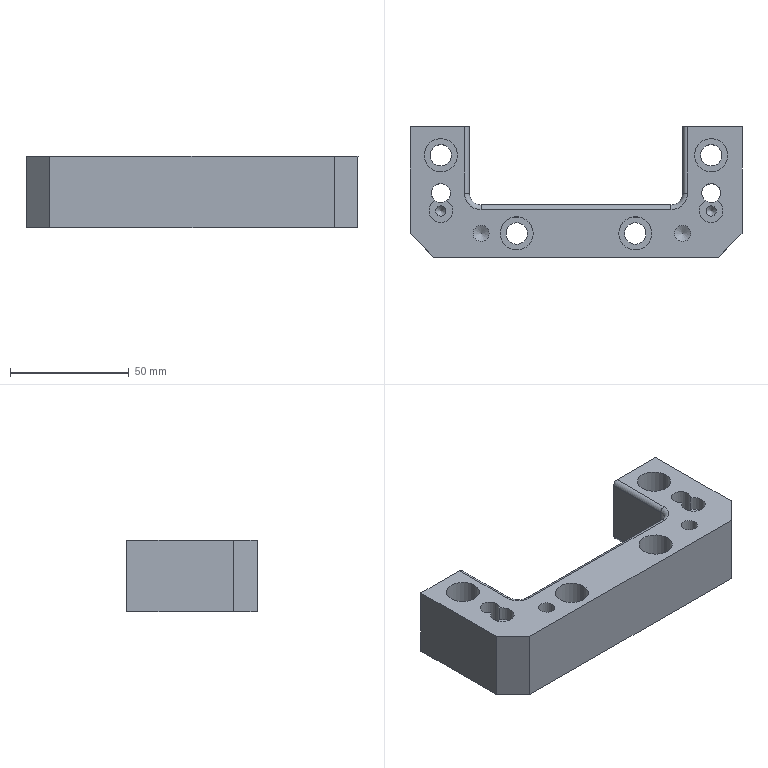Part | NX | features PS-20 2 | 1 solid | 50 faces | box 140 x 55 x 30 mm | volume 121432 mm3 | cylinder 24 | plane 18 | torus 4 | cone 4 | commonest cylinder face diameters 4 x6 9 x4 14 x4 4.306 x2 6.806 x2 8 x2
STEP:
#1=CARTESIAN_POINT('',(3232.594,-764.122,885.716));
#2=VERTEX_POINT('',#1);
#3=CARTESIAN_POINT('',(3232.594,-719.122,885.716));
#4=VERTEX_POINT('',#3);
#5=CARTESIAN_POINT('',(3232.594,-727.122,885.716));
#6=DIRECTION('',(0.,1.,0.));
#7=VECTOR('',#6,1000.);
#8=LINE('',#5,#7);
#9=EDGE_CURVE('',#2,#4,#8,.T.);
#10=ORIENTED_EDGE('',*,*,#9,.T.);
#11=CARTESIAN_POINT('',(3232.594,-719.122,915.716));
#12=VERTEX_POINT('',#11);
#13=CARTESIAN_POINT('',(3232.594,-719.122,900.716));
#14=DIRECTION('',(0.,0.,-1.));
#15=VECTOR('',#14,1000.);
#16=LINE('',#13,#15);
#17=EDGE_CURVE('',#12,#4,#16,.T.);
#18=ORIENTED_EDGE('',*,*,#17,.F.);
#19=CARTESIAN_POINT('',(3232.594,-764.122,915.716));
#20=VERTEX_POINT('',#19);
#21=CARTESIAN_POINT('',(3232.594,-727.122,915.716));
#22=DIRECTION('',(0.,1.,0.));
#23=VECTOR('',#22,1000.);
#24=LINE('',#21,#23);
#25=EDGE_CURVE('',#20,#12,#24,.T.);
#26=ORIENTED_EDGE('',*,*,#25,.F.);
#27=CARTESIAN_POINT('',(3232.594,-764.122,870.716));
#28=DIRECTION('',(0.,0.,1.));
#29=VECTOR('',#28,1000.);
#30=LINE('',#27,#29);
#31=EDGE_CURVE('',#2,#20,#30,.T.);
#32=ORIENTED_EDGE('',*,*,#31,.F.);
#33=EDGE_LOOP('',(#10,#18,#26,#32));
#34=FACE_BOUND('',#33,.T.);
#35=CARTESIAN_POINT('',(3232.594,-727.122,870.716));
#36=DIRECTION('',(1.,0.,0.));
#37=DIRECTION('',(0.,0.,-1.));
#38=AXIS2_PLACEMENT_3D('',#35,#36,#37);
#39=PLANE('',#38);
#40=ADVANCED_FACE('',(#34),#39,.T.);
#41=CARTESIAN_POINT('',(3207.594,-719.122,913.716));
#42=VERTEX_POINT('',#41);
#43=CARTESIAN_POINT('',(3207.594,-719.122,887.716));
#44=VERTEX_POINT('',#43);
#45=CARTESIAN_POINT('',(3207.594,-719.122,900.716));
#46=DIRECTION('',(0.,0.,-1.));
#47=VECTOR('',#46,1000.);
#48=LINE('',#45,#47);
#49=EDGE_CURVE('',#42,#44,#48,.T.);
#50=ORIENTED_EDGE('',*,*,#49,.T.);
#51=CARTESIAN_POINT('',(3207.594,-747.122,887.716));
#52=VERTEX_POINT('',#51);
#53=CARTESIAN_POINT('',(3207.594,-722.122,887.716));
#54=DIRECTION('',(0.,1.,0.));
#55=VECTOR('',#54,1000.);
#56=LINE('',#53,#55);
#57=EDGE_CURVE('',#52,#44,#56,.T.);
#58=ORIENTED_EDGE('',*,*,#57,.F.);
#59=CARTESIAN_POINT('',(3207.594,-747.122,913.716));
#60=VERTEX_POINT('',#59);
#61=CARTESIAN_POINT('',(3207.594,-747.122,890.716));
#62=DIRECTION('',(0.,0.,-1.));
#63=VECTOR('',#62,1000.);
#64=LINE('',#61,#63);
#65=EDGE_CURVE('',#60,#52,#64,.T.);
#66=ORIENTED_EDGE('',*,*,#65,.F.);
#67=CARTESIAN_POINT('',(3207.594,-747.122,913.716));
#68=DIRECTION('',(0.,-1.,0.));
#69=VECTOR('',#68,1000.);
#70=LINE('',#67,#69);
#71=EDGE_CURVE('',#42,#60,#70,.T.);
#72=ORIENTED_EDGE('',*,*,#71,.F.);
#73=EDGE_LOOP('',(#50,#58,#66,#72));
#74=FACE_BOUND('',#73,.T.);
#75=CARTESIAN_POINT('',(3207.594,-727.122,870.716));
#76=DIRECTION('',(1.,0.,0.));
#77=DIRECTION('',(0.,0.,-1.));
#78=AXIS2_PLACEMENT_3D('',#75,#76,#77);
#79=PLANE('',#78);
#80=ADVANCED_FACE('',(#74),#79,.F.);
#81=CARTESIAN_POINT('',(3117.594,-719.122,887.716));
#82=VERTEX_POINT('',#81);
#83=CARTESIAN_POINT('',(3117.594,-747.122,887.716));
#84=VERTEX_POINT('',#83);
#85=CARTESIAN_POINT('',(3117.594,-727.122,887.716));
#86=DIRECTION('',(0.,-1.,0.));
#87=VECTOR('',#86,1000.);
#88=LINE('',#85,#87);
#89=EDGE_CURVE('',#82,#84,#88,.T.);
#90=ORIENTED_EDGE('',*,*,#89,.F.);
#91=CARTESIAN_POINT('',(3117.594,-719.122,913.716));
#92=VERTEX_POINT('',#91);
#93=CARTESIAN_POINT('',(3117.594,-719.122,900.716));
#94=DIRECTION('',(0.,0.,-1.));
#95=VECTOR('',#94,1000.);
#96=LINE('',#93,#95);
#97=EDGE_CURVE('',#92,#82,#96,.T.);
#98=ORIENTED_EDGE('',*,*,#97,.F.);
#99=CARTESIAN_POINT('',(3117.594,-747.122,913.716));
#100=VERTEX_POINT('',#99);
#101=CARTESIAN_POINT('',(3117.594,-727.122,913.716));
#102=DIRECTION('',(0.,1.,0.));
#103=VECTOR('',#102,1000.);
#104=LINE('',#101,#103);
#105=EDGE_CURVE('',#100,#92,#104,.T.);
#106=ORIENTED_EDGE('',*,*,#105,.F.);
#107=CARTESIAN_POINT('',(3117.594,-747.122,870.716));
#108=DIRECTION('',(0.,0.,1.));
#109=VECTOR('',#108,1000.);
#110=LINE('',#107,#109);
#111=EDGE_CURVE('',#84,#100,#110,.T.);
#112=ORIENTED_EDGE('',*,*,#111,.F.);
#113=EDGE_LOOP('',(#90,#98,#106,#112));
#114=FACE_BOUND('',#113,.T.);
#115=CARTESIAN_POINT('',(3117.594,-727.122,870.716));
#116=DIRECTION('',(1.,0.,0.));
#117=DIRECTION('',(0.,0.,-1.));
#118=AXIS2_PLACEMENT_3D('',#115,#116,#117);
#119=PLANE('',#118);
#120=ADVANCED_FACE('',(#114),#119,.T.);
#121=CARTESIAN_POINT('',(3092.594,-719.122,915.716));
#122=VERTEX_POINT('',#121);
#123=CARTESIAN_POINT('',(3092.594,-719.122,885.716));
#124=VERTEX_POINT('',#123);
#125=CARTESIAN_POINT('',(3092.594,-719.122,900.716));
#126=DIRECTION('',(0.,0.,-1.));
#127=VECTOR('',#126,1000.);
#128=LINE('',#125,#127);
#129=EDGE_CURVE('',#122,#124,#128,.T.);
#130=ORIENTED_EDGE('',*,*,#129,.T.);
#131=CARTESIAN_POINT('',(3092.594,-764.122,885.716));
#132=VERTEX_POINT('',#131);
#133=CARTESIAN_POINT('',(3092.594,-727.122,885.716));
#134=DIRECTION('',(0.,1.,0.));
#135=VECTOR('',#134,1000.);
#136=LINE('',#133,#135);
#137=EDGE_CURVE('',#132,#124,#136,.T.);
#138=ORIENTED_EDGE('',*,*,#137,.F.);
#139=CARTESIAN_POINT('',(3092.594,-764.122,915.716));
#140=VERTEX_POINT('',#139);
#141=CARTESIAN_POINT('',(3092.594,-764.122,885.716));
#142=DIRECTION('',(0.,0.,-1.));
#143=VECTOR('',#142,1000.);
#144=LINE('',#141,#143);
#145=EDGE_CURVE('',#140,#132,#144,.T.);
#146=ORIENTED_EDGE('',*,*,#145,.F.);
#147=CARTESIAN_POINT('',(3092.594,-727.122,915.716));
#148=DIRECTION('',(0.,1.,0.));
#149=VECTOR('',#148,1000.);
#150=LINE('',#147,#149);
#151=EDGE_CURVE('',#140,#122,#150,.T.);
#152=ORIENTED_EDGE('',*,*,#151,.T.);
#153=EDGE_LOOP('',(#130,#138,#146,#152));
#154=FACE_BOUND('',#153,.T.);
#155=CARTESIAN_POINT('',(3092.594,-727.122,870.716));
#156=DIRECTION('',(1.,0.,0.));
#157=DIRECTION('',(0.,0.,-1.));
#158=AXIS2_PLACEMENT_3D('',#155,#156,#157);
#159=PLANE('',#158);
#160=ADVANCED_FACE('',(#154),#159,.F.);
#161=CARTESIAN_POINT('',(3109.594,-747.122,885.716));
#162=VERTEX_POINT('',#161);
#163=CARTESIAN_POINT('',(3105.594,-747.122,885.716));
#164=DIRECTION('',(0.,0.,1.));
#165=DIRECTION('',(1.,0.,0.));
#166=AXIS2_PLACEMENT_3D('',#163,#164,#165);
#167=CIRCLE('',#166,4.);
#168=EDGE_CURVE('',#162,#162,#167,.T.);
#169=ORIENTED_EDGE('',*,*,#168,.T.);
#170=EDGE_LOOP('',(#169));
#171=FACE_BOUND('',#170,.T.);
#172=CARTESIAN_POINT('',(3223.594,-747.122,885.716));
#173=VERTEX_POINT('',#172);
#174=CARTESIAN_POINT('',(3219.594,-747.122,885.716));
#175=DIRECTION('',(0.,0.,1.));
#176=DIRECTION('',(1.,0.,0.));
#177=AXIS2_PLACEMENT_3D('',#174,#175,#176);
#178=CIRCLE('',#177,4.);
#179=EDGE_CURVE('',#173,#173,#178,.T.);
#180=ORIENTED_EDGE('',*,*,#179,.T.);
#181=EDGE_LOOP('',(#180));
#182=FACE_BOUND('',#181,.T.);
#183=CARTESIAN_POINT('',(3192.094,-764.122,885.716));
#184=VERTEX_POINT('',#183);
#185=CARTESIAN_POINT('',(3187.594,-764.122,885.716));
#186=DIRECTION('',(0.,0.,1.));
#187=DIRECTION('',(1.,0.,0.));
#188=AXIS2_PLACEMENT_3D('',#185,#186,#187);
#189=CIRCLE('',#188,4.5);
#190=EDGE_CURVE('',#184,#184,#189,.T.);
#191=ORIENTED_EDGE('',*,*,#190,.T.);
#192=EDGE_LOOP('',(#191));
#193=FACE_BOUND('',#192,.T.);
#194=CARTESIAN_POINT('',(3142.094,-764.122,885.716));
#195=VERTEX_POINT('',#194);
#196=CARTESIAN_POINT('',(3137.594,-764.122,885.716));
#197=DIRECTION('',(0.,0.,1.));
#198=DIRECTION('',(1.,0.,0.));
#199=AXIS2_PLACEMENT_3D('',#196,#197,#198);
#200=CIRCLE('',#199,4.5);
#201=EDGE_CURVE('',#195,#195,#200,.T.);
#202=ORIENTED_EDGE('',*,*,#201,.T.);
#203=EDGE_LOOP('',(#202));
#204=FACE_BOUND('',#203,.T.);
#205=CARTESIAN_POINT('',(3110.094,-731.122,885.716));
#206=VERTEX_POINT('',#205);
#207=CARTESIAN_POINT('',(3105.594,-731.122,885.716));
#208=DIRECTION('',(0.,0.,1.));
#209=DIRECTION('',(1.,0.,0.));
#210=AXIS2_PLACEMENT_3D('',#207,#208,#209);
#211=CIRCLE('',#210,4.5);
#212=EDGE_CURVE('',#206,#206,#211,.T.);
#213=ORIENTED_EDGE('',*,*,#212,.T.);
#214=EDGE_LOOP('',(#213));
#215=FACE_BOUND('',#214,.T.);
#216=CARTESIAN_POINT('',(3224.094,-731.122,885.716));
#217=VERTEX_POINT('',#216);
#218=CARTESIAN_POINT('',(3219.594,-731.122,885.716));
#219=DIRECTION('',(0.,0.,1.));
#220=DIRECTION('',(1.,0.,0.));
#221=AXIS2_PLACEMENT_3D('',#218,#219,#220);
#222=CIRCLE('',#221,4.5);
#223=EDGE_CURVE('',#217,#217,#222,.T.);
#224=ORIENTED_EDGE('',*,*,#223,.T.);
#225=EDGE_LOOP('',(#224));
#226=FACE_BOUND('',#225,.T.);
#227=CARTESIAN_POINT('',(3209.594,-719.122,885.716));
#228=VERTEX_POINT('',#227);
#229=CARTESIAN_POINT('',(3105.094,-719.122,885.716));
#230=DIRECTION('',(1.,0.,0.));
#231=VECTOR('',#230,1000.);
#232=LINE('',#229,#231);
#233=EDGE_CURVE('',#228,#4,#232,.T.);
#234=ORIENTED_EDGE('',*,*,#233,.T.);
#235=ORIENTED_EDGE('',*,*,#9,.F.);
#236=CARTESIAN_POINT('',(3222.594,-774.122,885.716));
#237=VERTEX_POINT('',#236);
#238=CARTESIAN_POINT('',(3190.094,-806.622,885.716));
#239=DIRECTION('',(0.7071,0.7071,0.));
#240=VECTOR('',#239,1000.);
#241=LINE('',#238,#240);
#242=EDGE_CURVE('',#237,#2,#241,.T.);
#243=ORIENTED_EDGE('',*,*,#242,.F.);
#244=CARTESIAN_POINT('',(3102.594,-774.122,885.716));
#245=VERTEX_POINT('',#244);
#246=CARTESIAN_POINT('',(3112.594,-774.122,885.716));
#247=DIRECTION('',(1.,0.,0.));
#248=VECTOR('',#247,1000.);
#249=LINE('',#246,#248);
#250=EDGE_CURVE('',#245,#237,#249,.T.);
#251=ORIENTED_EDGE('',*,*,#250,.F.);
#252=CARTESIAN_POINT('',(3085.094,-756.622,885.716));
#253=DIRECTION('',(0.7071,-0.7071,0.));
#254=VECTOR('',#253,1000.);
#255=LINE('',#252,#254);
#256=EDGE_CURVE('',#132,#245,#255,.T.);
#257=ORIENTED_EDGE('',*,*,#256,.F.);
#258=ORIENTED_EDGE('',*,*,#137,.T.);
#259=CARTESIAN_POINT('',(3115.594,-719.122,885.716));
#260=VERTEX_POINT('',#259);
#261=CARTESIAN_POINT('',(3105.094,-719.122,885.716));
#262=DIRECTION('',(1.,0.,0.));
#263=VECTOR('',#262,1000.);
#264=LINE('',#261,#263);
#265=EDGE_CURVE('',#124,#260,#264,.T.);
#266=ORIENTED_EDGE('',*,*,#265,.T.);
#267=CARTESIAN_POINT('',(3115.594,-747.122,885.716));
#268=VERTEX_POINT('',#267);
#269=CARTESIAN_POINT('',(3115.594,-727.122,885.716));
#270=DIRECTION('',(0.,1.,0.));
#271=VECTOR('',#270,1000.);
#272=LINE('',#269,#271);
#273=EDGE_CURVE('',#268,#260,#272,.T.);
#274=ORIENTED_EDGE('',*,*,#273,.F.);
#275=CARTESIAN_POINT('',(3122.594,-754.122,885.716));
#276=VERTEX_POINT('',#275);
#277=CARTESIAN_POINT('',(3122.594,-747.122,885.716));
#278=DIRECTION('',(0.,0.,-1.));
#279=DIRECTION('',(1.,0.,0.));
#280=AXIS2_PLACEMENT_3D('',#277,#278,#279);
#281=CIRCLE('',#280,7.);
#282=EDGE_CURVE('',#276,#268,#281,.T.);
#283=ORIENTED_EDGE('',*,*,#282,.F.);
#284=CARTESIAN_POINT('',(3202.594,-754.122,885.716));
#285=VERTEX_POINT('',#284);
#286=CARTESIAN_POINT('',(3117.594,-754.122,885.716));
#287=DIRECTION('',(-1.,0.,0.));
#288=VECTOR('',#287,1000.);
#289=LINE('',#286,#288);
#290=EDGE_CURVE('',#285,#276,#289,.T.);
#291=ORIENTED_EDGE('',*,*,#290,.F.);
#292=CARTESIAN_POINT('',(3209.594,-747.122,885.716));
#293=VERTEX_POINT('',#292);
#294=CARTESIAN_POINT('',(3202.594,-747.122,885.716));
#295=DIRECTION('',(0.,0.,-1.));
#296=DIRECTION('',(1.,0.,0.));
#297=AXIS2_PLACEMENT_3D('',#294,#295,#296);
#298=CIRCLE('',#297,7.);
#299=EDGE_CURVE('',#293,#285,#298,.T.);
#300=ORIENTED_EDGE('',*,*,#299,.F.);
#301=CARTESIAN_POINT('',(3209.594,-727.122,885.716));
#302=DIRECTION('',(0.,-1.,0.));
#303=VECTOR('',#302,1000.);
#304=LINE('',#301,#303);
#305=EDGE_CURVE('',#228,#293,#304,.T.);
#306=ORIENTED_EDGE('',*,*,#305,.F.);
#307=EDGE_LOOP('',(#234,#235,#243,#251,#257,#258,#266,#274,#283,#291,#300,#306));
#308=FACE_BOUND('',#307,.T.);
#309=CARTESIAN_POINT('',(3112.594,-727.122,885.716));
#310=DIRECTION('',(0.,0.,1.));
#311=DIRECTION('',(0.,1.,0.));
#312=AXIS2_PLACEMENT_3D('',#309,#310,#311);
#313=PLANE('',#312);
#314=ADVANCED_FACE('',(#171,#182,#193,#204,#215,#226,#308),#313,.F.);
#315=CARTESIAN_POINT('',(3204.191,-764.122,915.716));
#316=VERTEX_POINT('',#315);
#317=CARTESIAN_POINT('',(3207.594,-764.122,915.716));
#318=DIRECTION('',(0.,0.,-1.));
#319=DIRECTION('',(-1.,0.,0.));
#320=AXIS2_PLACEMENT_3D('',#317,#318,#319);
#321=CIRCLE('',#320,3.403);
#322=EDGE_CURVE('',#316,#316,#321,.T.);
#323=ORIENTED_EDGE('',*,*,#322,.T.);
#324=EDGE_LOOP('',(#323));
#325=FACE_BOUND('',#324,.T.);
#326=CARTESIAN_POINT('',(3119.191,-764.122,915.716));
#327=VERTEX_POINT('',#326);
#328=CARTESIAN_POINT('',(3122.594,-764.122,915.716));
#329=DIRECTION('',(0.,0.,-1.));
#330=DIRECTION('',(-1.,0.,0.));
#331=AXIS2_PLACEMENT_3D('',#328,#329,#330);
#332=CIRCLE('',#331,3.403);
#333=EDGE_CURVE('',#327,#327,#332,.T.);
#334=ORIENTED_EDGE('',*,*,#333,.T.);
#335=EDGE_LOOP('',(#334));
#336=FACE_BOUND('',#335,.T.);
#337=CARTESIAN_POINT('',(3103.125,-750.269,915.716));
#338=VERTEX_POINT('',#337);
#339=CARTESIAN_POINT('',(3108.063,-750.269,915.716));
#340=VERTEX_POINT('',#339);
#341=CARTESIAN_POINT('',(3105.594,-747.122,915.716));
#342=DIRECTION('',(0.,0.,1.));
#343=DIRECTION('',(1.,0.,0.));
#344=AXIS2_PLACEMENT_3D('',#341,#342,#343);
#345=CIRCLE('',#344,4.);
#346=EDGE_CURVE('',#338,#340,#345,.F.);
#347=ORIENTED_EDGE('',*,*,#346,.T.);
#348=CARTESIAN_POINT('',(3105.594,-754.622,915.716));
#349=DIRECTION('',(0.,0.,-1.));
#350=DIRECTION('',(-0.9185,0.3955,0.));
#351=AXIS2_PLACEMENT_3D('',#348,#349,#350);
#352=CIRCLE('',#351,5.004);
#353=EDGE_CURVE('',#340,#338,#352,.T.);
#354=ORIENTED_EDGE('',*,*,#353,.T.);
#355=EDGE_LOOP('',(#347,#354));
#356=FACE_BOUND('',#355,.T.);
#357=CARTESIAN_POINT('',(3194.594,-764.122,915.716));
#358=VERTEX_POINT('',#357);
#359=CARTESIAN_POINT('',(3187.594,-764.122,915.716));
#360=DIRECTION('',(0.,0.,-1.));
#361=DIRECTION('',(1.,0.,0.));
#362=AXIS2_PLACEMENT_3D('',#359,#360,#361);
#363=CIRCLE('',#362,7.);
#364=EDGE_CURVE('',#358,#358,#363,.T.);
#365=ORIENTED_EDGE('',*,*,#364,.T.);
#366=EDGE_LOOP('',(#365));
#367=FACE_BOUND('',#366,.T.);
#368=CARTESIAN_POINT('',(3130.594,-764.122,915.716));
#369=VERTEX_POINT('',#368);
#370=CARTESIAN_POINT('',(3137.594,-764.122,915.716));
#371=DIRECTION('',(0.,0.,1.));
#372=DIRECTION('',(1.,0.,0.));
#373=AXIS2_PLACEMENT_3D('',#370,#371,#372);
#374=CIRCLE('',#373,7.);
#375=EDGE_CURVE('',#369,#369,#374,.T.);
#376=ORIENTED_EDGE('',*,*,#375,.F.);
#377=EDGE_LOOP('',(#376));
#378=FACE_BOUND('',#377,.T.);
#379=CARTESIAN_POINT('',(3112.594,-731.122,915.716));
#380=VERTEX_POINT('',#379);
#381=CARTESIAN_POINT('',(3105.594,-731.122,915.716));
#382=DIRECTION('',(0.,0.,-1.));
#383=DIRECTION('',(1.,0.,0.));
#384=AXIS2_PLACEMENT_3D('',#381,#382,#383);
#385=CIRCLE('',#384,7.);
#386=EDGE_CURVE('',#380,#380,#385,.T.);
#387=ORIENTED_EDGE('',*,*,#386,.T.);
#388=EDGE_LOOP('',(#387));
#389=FACE_BOUND('',#388,.T.);
#390=CARTESIAN_POINT('',(3212.594,-731.122,915.716));
#391=VERTEX_POINT('',#390);
#392=CARTESIAN_POINT('',(3219.594,-731.122,915.716));
#393=DIRECTION('',(0.,0.,1.));
#394=DIRECTION('',(1.,0.,0.));
#395=AXIS2_PLACEMENT_3D('',#392,#393,#394);
#396=CIRCLE('',#395,7.);
#397=EDGE_CURVE('',#391,#391,#396,.T.);
#398=ORIENTED_EDGE('',*,*,#397,.F.);
#399=EDGE_LOOP('',(#398));
#400=FACE_BOUND('',#399,.T.);
#401=CARTESIAN_POINT('',(3217.125,-750.269,915.716));
#402=VERTEX_POINT('',#401);
#403=CARTESIAN_POINT('',(3222.063,-750.269,915.716));
#404=VERTEX_POINT('',#403);
#405=CARTESIAN_POINT('',(3219.594,-747.122,915.716));
#406=DIRECTION('',(0.,0.,1.));
#407=DIRECTION('',(1.,0.,0.));
#408=AXIS2_PLACEMENT_3D('',#405,#406,#407);
#409=CIRCLE('',#408,4.);
#410=EDGE_CURVE('',#402,#404,#409,.F.);
#411=ORIENTED_EDGE('',*,*,#410,.T.);
#412=CARTESIAN_POINT('',(3219.594,-754.622,915.716));
#413=DIRECTION('',(0.,0.,-1.));
#414=DIRECTION('',(-0.9185,0.3955,0.));
#415=AXIS2_PLACEMENT_3D('',#412,#413,#414);
#416=CIRCLE('',#415,5.004);
#417=EDGE_CURVE('',#404,#402,#416,.T.);
#418=ORIENTED_EDGE('',*,*,#417,.T.);
#419=EDGE_LOOP('',(#411,#418));
#420=FACE_BOUND('',#419,.T.);
#421=ORIENTED_EDGE('',*,*,#25,.T.);
#422=CARTESIAN_POINT('',(3209.594,-719.122,915.716));
#423=VERTEX_POINT('',#422);
#424=CARTESIAN_POINT('',(3375.094,-719.122,915.716));
#425=DIRECTION('',(-1.,0.,0.));
#426=VECTOR('',#425,1000.);
#427=LINE('',#424,#426);
#428=EDGE_CURVE('',#12,#423,#427,.T.);
#429=ORIENTED_EDGE('',*,*,#428,.T.);
#430=CARTESIAN_POINT('',(3209.594,-747.122,915.716));
#431=VERTEX_POINT('',#430);
#432=CARTESIAN_POINT('',(3209.594,-862.122,915.716));
#433=DIRECTION('',(0.,1.,0.));
#434=VECTOR('',#433,1000.);
#435=LINE('',#432,#434);
#436=EDGE_CURVE('',#431,#423,#435,.T.);
#437=ORIENTED_EDGE('',*,*,#436,.F.);
#438=CARTESIAN_POINT('',(3202.594,-754.122,915.716));
#439=VERTEX_POINT('',#438);
#440=CARTESIAN_POINT('',(3202.594,-747.122,915.716));
#441=DIRECTION('',(0.,0.,1.));
#442=DIRECTION('',(1.,0.,0.));
#443=AXIS2_PLACEMENT_3D('',#440,#441,#442);
#444=CIRCLE('',#443,7.);
#445=EDGE_CURVE('',#439,#431,#444,.T.);
#446=ORIENTED_EDGE('',*,*,#445,.F.);
#447=CARTESIAN_POINT('',(3122.594,-754.122,915.716));
#448=VERTEX_POINT('',#447);
#449=CARTESIAN_POINT('',(3207.594,-754.122,915.716));
#450=DIRECTION('',(1.,0.,0.));
#451=VECTOR('',#450,1000.);
#452=LINE('',#449,#451);
#453=EDGE_CURVE('',#448,#439,#452,.T.);
#454=ORIENTED_EDGE('',*,*,#453,.F.);
#455=CARTESIAN_POINT('',(3115.594,-747.122,915.716));
#456=VERTEX_POINT('',#455);
#457=CARTESIAN_POINT('',(3122.594,-747.122,915.716));
#458=DIRECTION('',(0.,0.,1.));
#459=DIRECTION('',(1.,0.,0.));
#460=AXIS2_PLACEMENT_3D('',#457,#458,#459);
#461=CIRCLE('',#460,7.);
#462=EDGE_CURVE('',#456,#448,#461,.T.);
#463=ORIENTED_EDGE('',*,*,#462,.F.);
#464=CARTESIAN_POINT('',(3115.594,-719.122,915.716));
#465=VERTEX_POINT('',#464);
#466=CARTESIAN_POINT('',(3115.594,-862.122,915.716));
#467=DIRECTION('',(0.,-1.,0.));
#468=VECTOR('',#467,1000.);
#469=LINE('',#466,#468);
#470=EDGE_CURVE('',#465,#456,#469,.T.);
#471=ORIENTED_EDGE('',*,*,#470,.F.);
#472=CARTESIAN_POINT('',(3375.094,-719.122,915.716));
#473=DIRECTION('',(-1.,0.,0.));
#474=VECTOR('',#473,1000.);
#475=LINE('',#472,#474);
#476=EDGE_CURVE('',#465,#122,#475,.T.);
#477=ORIENTED_EDGE('',*,*,#476,.T.);
#478=ORIENTED_EDGE('',*,*,#151,.F.);
#479=CARTESIAN_POINT('',(3102.594,-774.122,915.716));
#480=VERTEX_POINT('',#479);
#481=CARTESIAN_POINT('',(3092.594,-764.122,915.716));
#482=DIRECTION('',(-0.7071,0.7071,0.));
#483=VECTOR('',#482,1000.);
#484=LINE('',#481,#483);
#485=EDGE_CURVE('',#480,#140,#484,.T.);
#486=ORIENTED_EDGE('',*,*,#485,.F.);
#487=CARTESIAN_POINT('',(3222.594,-774.122,915.716));
#488=VERTEX_POINT('',#487);
#489=CARTESIAN_POINT('',(3375.094,-774.122,915.716));
#490=DIRECTION('',(1.,0.,0.));
#491=VECTOR('',#490,1000.);
#492=LINE('',#489,#491);
#493=EDGE_CURVE('',#480,#488,#492,.T.);
#494=ORIENTED_EDGE('',*,*,#493,.T.);
#495=CARTESIAN_POINT('',(3256.344,-740.372,915.716));
#496=DIRECTION('',(-0.7071,-0.7071,0.));
#497=VECTOR('',#496,1000.);
#498=LINE('',#495,#497);
#499=EDGE_CURVE('',#20,#488,#498,.T.);
#500=ORIENTED_EDGE('',*,*,#499,.F.);
#501=EDGE_LOOP('',(#421,#429,#437,#446,#454,#463,#471,#477,#478,#486,#494,#500));
#502=FACE_BOUND('',#501,.T.);
#503=CARTESIAN_POINT('',(3375.094,-862.122,915.716));
#504=DIRECTION('',(0.,0.,1.));
#505=DIRECTION('',(0.,-1.,0.));
#506=AXIS2_PLACEMENT_3D('',#503,#504,#505);
#507=PLANE('',#506);
#508=ADVANCED_FACE('',(#325,#336,#356,#367,#378,#389,#400,#420,#502),#507,.T.);
#509=ORIENTED_EDGE('',*,*,#436,.T.);
#510=CARTESIAN_POINT('',(3209.594,-719.122,913.716));
#511=DIRECTION('',(0.,1.,0.));
#512=DIRECTION('',(0.,0.,1.));
#513=AXIS2_PLACEMENT_3D('',#510,#511,#512);
#514=CIRCLE('',#513,2.);
#515=EDGE_CURVE('',#423,#42,#514,.F.);
#516=ORIENTED_EDGE('',*,*,#515,.T.);
#517=ORIENTED_EDGE('',*,*,#71,.T.);
#518=CARTESIAN_POINT('',(3209.594,-747.122,913.716));
#519=DIRECTION('',(0.,1.,0.));
#520=DIRECTION('',(0.,0.,-1.));
#521=AXIS2_PLACEMENT_3D('',#518,#519,#520);
#522=CIRCLE('',#521,2.);
#523=EDGE_CURVE('',#60,#431,#522,.T.);
#524=ORIENTED_EDGE('',*,*,#523,.T.);
#525=EDGE_LOOP('',(#509,#516,#517,#524));
#526=FACE_BOUND('',#525,.T.);
#527=CARTESIAN_POINT('',(3209.594,-862.122,913.716));
#528=DIRECTION('',(0.,-1.,0.));
#529=DIRECTION('',(0.,0.,1.));
#530=AXIS2_PLACEMENT_3D('',#527,#528,#529);
#531=CYLINDRICAL_SURFACE('',#530,2.);
#532=ADVANCED_FACE('',(#526),#531,.T.);
#533=ORIENTED_EDGE('',*,*,#105,.T.);
#534=CARTESIAN_POINT('',(3115.594,-719.122,913.716));
#535=DIRECTION('',(0.,1.,0.));
#536=DIRECTION('',(0.,0.,1.));
#537=AXIS2_PLACEMENT_3D('',#534,#535,#536);
#538=CIRCLE('',#537,2.);
#539=EDGE_CURVE('',#465,#92,#538,.T.);
#540=ORIENTED_EDGE('',*,*,#539,.F.);
#541=ORIENTED_EDGE('',*,*,#470,.T.);
#542=CARTESIAN_POINT('',(3115.594,-747.122,913.716));
#543=DIRECTION('',(0.,-1.,0.));
#544=DIRECTION('',(0.,0.,1.));
#545=AXIS2_PLACEMENT_3D('',#542,#543,#544);
#546=CIRCLE('',#545,2.);
#547=EDGE_CURVE('',#100,#456,#546,.T.);
#548=ORIENTED_EDGE('',*,*,#547,.F.);
#549=EDGE_LOOP('',(#533,#540,#541,#548));
#550=FACE_BOUND('',#549,.T.);
#551=CARTESIAN_POINT('',(3115.594,-727.122,913.716));
#552=DIRECTION('',(0.,1.,0.));
#553=DIRECTION('',(0.,0.,-1.));
#554=AXIS2_PLACEMENT_3D('',#551,#552,#553);
#555=CYLINDRICAL_SURFACE('',#554,2.);
#556=ADVANCED_FACE('',(#550),#555,.T.);
#557=ORIENTED_EDGE('',*,*,#57,.T.);
#558=CARTESIAN_POINT('',(3209.594,-719.122,887.716));
#559=DIRECTION('',(0.,1.,0.));
#560=DIRECTION('',(0.,0.,1.));
#561=AXIS2_PLACEMENT_3D('',#558,#559,#560);
#562=CIRCLE('',#561,2.);
#563=EDGE_CURVE('',#228,#44,#562,.T.);
#564=ORIENTED_EDGE('',*,*,#563,.F.);
#565=ORIENTED_EDGE('',*,*,#305,.T.);
#566=CARTESIAN_POINT('',(3209.594,-747.122,887.716));
#567=DIRECTION('',(0.,1.,0.));
#568=DIRECTION('',(0.,0.,1.));
#569=AXIS2_PLACEMENT_3D('',#566,#567,#568);
#570=CIRCLE('',#569,2.);
#571=EDGE_CURVE('',#293,#52,#570,.T.);
#572=ORIENTED_EDGE('',*,*,#571,.T.);
#573=EDGE_LOOP('',(#557,#564,#565,#572));
#574=FACE_BOUND('',#573,.T.);
#575=CARTESIAN_POINT('',(3209.594,-727.122,887.716));
#576=DIRECTION('',(0.,1.,0.));
#577=DIRECTION('',(0.,0.,-1.));
#578=AXIS2_PLACEMENT_3D('',#575,#576,#577);
#579=CYLINDRICAL_SURFACE('',#578,2.);
#580=ADVANCED_FACE('',(#574),#579,.T.);
#581=ORIENTED_EDGE('',*,*,#273,.T.);
#582=CARTESIAN_POINT('',(3115.594,-719.122,887.716));
#583=DIRECTION('',(0.,1.,0.));
#584=DIRECTION('',(0.,0.,1.));
#585=AXIS2_PLACEMENT_3D('',#582,#583,#584);
#586=CIRCLE('',#585,2.);
#587=EDGE_CURVE('',#82,#260,#586,.T.);
#588=ORIENTED_EDGE('',*,*,#587,.F.);
#589=ORIENTED_EDGE('',*,*,#89,.T.);
#590=CARTESIAN_POINT('',(3115.594,-747.122,887.716));
#591=DIRECTION('',(0.,-1.,0.));
#592=DIRECTION('',(0.,0.,-1.));
#593=AXIS2_PLACEMENT_3D('',#590,#591,#592);
#594=CIRCLE('',#593,2.);
#595=EDGE_CURVE('',#268,#84,#594,.T.);
#596=ORIENTED_EDGE('',*,*,#595,.F.);
#597=EDGE_LOOP('',(#581,#588,#589,#596));
#598=FACE_BOUND('',#597,.T.);
#599=CARTESIAN_POINT('',(3115.594,-727.122,887.716));
#600=DIRECTION('',(0.,-1.,0.));
#601=DIRECTION('',(0.,0.,1.));
#602=AXIS2_PLACEMENT_3D('',#599,#600,#601);
#603=CYLINDRICAL_SURFACE('',#602,2.);
#604=ADVANCED_FACE('',(#598),#603,.T.);
#605=CARTESIAN_POINT('',(3215.094,-731.122,905.716));
#606=VERTEX_POINT('',#605);
#607=CARTESIAN_POINT('',(3219.594,-731.122,905.716));
#608=DIRECTION('',(0.,0.,-1.));
#609=DIRECTION('',(-1.,0.,0.));
#610=AXIS2_PLACEMENT_3D('',#607,#608,#609);
#611=CIRCLE('',#610,4.5);
#612=EDGE_CURVE('',#606,#606,#611,.T.);
#613=ORIENTED_EDGE('',*,*,#612,.T.);
#614=EDGE_LOOP('',(#613));
#615=FACE_BOUND('',#614,.T.);
#616=CARTESIAN_POINT('',(3212.594,-731.122,905.716));
#617=VERTEX_POINT('',#616);
#618=CARTESIAN_POINT('',(3219.594,-731.122,905.716));
#619=DIRECTION('',(0.,0.,-1.));
#620=DIRECTION('',(-1.,0.,0.));
#621=AXIS2_PLACEMENT_3D('',#618,#619,#620);
#622=CIRCLE('',#621,7.);
#623=EDGE_CURVE('',#617,#617,#622,.T.);
#624=ORIENTED_EDGE('',*,*,#623,.F.);
#625=EDGE_LOOP('',(#624));
#626=FACE_BOUND('',#625,.T.);
#627=CARTESIAN_POINT('',(3219.594,-731.122,905.716));
#628=DIRECTION('',(0.,0.,-1.));
#629=DIRECTION('',(-1.,0.,0.));
#630=AXIS2_PLACEMENT_3D('',#627,#628,#629);
#631=PLANE('',#630);
#632=ADVANCED_FACE('',(#615,#626),#631,.F.);
#633=CARTESIAN_POINT('',(3101.094,-731.122,905.716));
#634=VERTEX_POINT('',#633);
#635=CARTESIAN_POINT('',(3105.594,-731.122,905.716));
#636=DIRECTION('',(0.,0.,-1.));
#637=DIRECTION('',(-1.,0.,0.));
#638=AXIS2_PLACEMENT_3D('',#635,#636,#637);
#639=CIRCLE('',#638,4.5);
#640=EDGE_CURVE('',#634,#634,#639,.T.);
#641=ORIENTED_EDGE('',*,*,#640,.T.);
#642=EDGE_LOOP('',(#641));
#643=FACE_BOUND('',#642,.T.);
#644=CARTESIAN_POINT('',(3098.594,-731.122,905.716));
#645=VERTEX_POINT('',#644);
#646=CARTESIAN_POINT('',(3105.594,-731.122,905.716));
#647=DIRECTION('',(0.,0.,-1.));
#648=DIRECTION('',(-1.,0.,0.));
#649=AXIS2_PLACEMENT_3D('',#646,#647,#648);
#650=CIRCLE('',#649,7.);
#651=EDGE_CURVE('',#645,#645,#650,.T.);
#652=ORIENTED_EDGE('',*,*,#651,.F.);
#653=EDGE_LOOP('',(#652));
#654=FACE_BOUND('',#653,.T.);
#655=CARTESIAN_POINT('',(3105.594,-731.122,905.716));
#656=DIRECTION('',(0.,0.,-1.));
#657=DIRECTION('',(1.,0.,0.));
#658=AXIS2_PLACEMENT_3D('',#655,#656,#657);
#659=PLANE('',#658);
#660=ADVANCED_FACE('',(#643,#654),#659,.F.);
#661=CARTESIAN_POINT('',(3133.094,-764.122,905.716));
#662=VERTEX_POINT('',#661);
#663=CARTESIAN_POINT('',(3137.594,-764.122,905.716));
#664=DIRECTION('',(0.,0.,-1.));
#665=DIRECTION('',(-1.,0.,0.));
#666=AXIS2_PLACEMENT_3D('',#663,#664,#665);
#667=CIRCLE('',#666,4.5);
#668=EDGE_CURVE('',#662,#662,#667,.T.);
#669=ORIENTED_EDGE('',*,*,#668,.T.);
#670=EDGE_LOOP('',(#669));
#671=FACE_BOUND('',#670,.T.);
#672=CARTESIAN_POINT('',(3130.594,-764.122,905.716));
#673=VERTEX_POINT('',#672);
#674=CARTESIAN_POINT('',(3137.594,-764.122,905.716));
#675=DIRECTION('',(0.,0.,-1.));
#676=DIRECTION('',(-1.,0.,0.));
#677=AXIS2_PLACEMENT_3D('',#674,#675,#676);
#678=CIRCLE('',#677,7.);
#679=EDGE_CURVE('',#673,#673,#678,.T.);
#680=ORIENTED_EDGE('',*,*,#679,.F.);
#681=EDGE_LOOP('',(#680));
#682=FACE_BOUND('',#681,.T.);
#683=CARTESIAN_POINT('',(3137.594,-764.122,905.716));
#684=DIRECTION('',(0.,0.,-1.));
#685=DIRECTION('',(-1.,0.,0.));
#686=AXIS2_PLACEMENT_3D('',#683,#684,#685);
#687=PLANE('',#686);
#688=ADVANCED_FACE('',(#671,#682),#687,.F.);
#689=CARTESIAN_POINT('',(3183.094,-764.122,905.716));
#690=VERTEX_POINT('',#689);
#691=CARTESIAN_POINT('',(3187.594,-764.122,905.716));
#692=DIRECTION('',(0.,0.,-1.));
#693=DIRECTION('',(-1.,0.,0.));
#694=AXIS2_PLACEMENT_3D('',#691,#692,#693);
#695=CIRCLE('',#694,4.5);
#696=EDGE_CURVE('',#690,#690,#695,.T.);
#697=ORIENTED_EDGE('',*,*,#696,.T.);
#698=EDGE_LOOP('',(#697));
#699=FACE_BOUND('',#698,.T.);
#700=CARTESIAN_POINT('',(3180.594,-764.122,905.716));
#701=VERTEX_POINT('',#700);
#702=CARTESIAN_POINT('',(3187.594,-764.122,905.716));
#703=DIRECTION('',(0.,0.,-1.));
#704=DIRECTION('',(-1.,0.,0.));
#705=AXIS2_PLACEMENT_3D('',#702,#703,#704);
#706=CIRCLE('',#705,7.);
#707=EDGE_CURVE('',#701,#701,#706,.T.);
#708=ORIENTED_EDGE('',*,*,#707,.F.);
#709=EDGE_LOOP('',(#708));
#710=FACE_BOUND('',#709,.T.);
#711=CARTESIAN_POINT('',(3187.594,-764.122,905.716));
#712=DIRECTION('',(0.,0.,-1.));
#713=DIRECTION('',(1.,0.,0.));
#714=AXIS2_PLACEMENT_3D('',#711,#712,#713);
#715=PLANE('',#714);
#716=ADVANCED_FACE('',(#699,#710),#715,.F.);
#717=ORIENTED_EDGE('',*,*,#223,.F.);
#718=EDGE_LOOP('',(#717));
#719=FACE_BOUND('',#718,.T.);
#720=ORIENTED_EDGE('',*,*,#612,.F.);
#721=EDGE_LOOP('',(#720));
#722=FACE_BOUND('',#721,.T.);
#723=CARTESIAN_POINT('',(3219.594,-731.122,785.716));
#724=DIRECTION('',(0.,0.,-1.));
#725=DIRECTION('',(-1.,0.,0.));
#726=AXIS2_PLACEMENT_3D('',#723,#724,#725);
#727=CYLINDRICAL_SURFACE('',#726,4.5);
#728=ADVANCED_FACE('',(#719,#722),#727,.F.);
#729=ORIENTED_EDGE('',*,*,#212,.F.);
#730=EDGE_LOOP('',(#729));
#731=FACE_BOUND('',#730,.T.);
#732=ORIENTED_EDGE('',*,*,#640,.F.);
#733=EDGE_LOOP('',(#732));
#734=FACE_BOUND('',#733,.T.);
#735=CARTESIAN_POINT('',(3105.594,-731.122,785.716));
#736=DIRECTION('',(0.,0.,-1.));
#737=DIRECTION('',(1.,0.,0.));
#738=AXIS2_PLACEMENT_3D('',#735,#736,#737);
#739=CYLINDRICAL_SURFACE('',#738,4.5);
#740=ADVANCED_FACE('',(#731,#734),#739,.F.);
#741=ORIENTED_EDGE('',*,*,#201,.F.);
#742=EDGE_LOOP('',(#741));
#743=FACE_BOUND('',#742,.T.);
#744=ORIENTED_EDGE('',*,*,#668,.F.);
#745=EDGE_LOOP('',(#744));
#746=FACE_BOUND('',#745,.T.);
#747=CARTESIAN_POINT('',(3137.594,-764.122,785.716));
#748=DIRECTION('',(0.,0.,-1.));
#749=DIRECTION('',(-1.,0.,0.));
#750=AXIS2_PLACEMENT_3D('',#747,#748,#749);
#751=CYLINDRICAL_SURFACE('',#750,4.5);
#752=ADVANCED_FACE('',(#743,#746),#751,.F.);
#753=ORIENTED_EDGE('',*,*,#190,.F.);
#754=EDGE_LOOP('',(#753));
#755=FACE_BOUND('',#754,.T.);
#756=ORIENTED_EDGE('',*,*,#696,.F.);
#757=EDGE_LOOP('',(#756));
#758=FACE_BOUND('',#757,.T.);
#759=CARTESIAN_POINT('',(3187.594,-764.122,785.716));
#760=DIRECTION('',(0.,0.,-1.));
#761=DIRECTION('',(1.,0.,0.));
#762=AXIS2_PLACEMENT_3D('',#759,#760,#761);
#763=CYLINDRICAL_SURFACE('',#762,4.5);
#764=ADVANCED_FACE('',(#755,#758),#763,.F.);
#765=ORIENTED_EDGE('',*,*,#179,.F.);
#766=EDGE_LOOP('',(#765));
#767=FACE_BOUND('',#766,.T.);
#768=ORIENTED_EDGE('',*,*,#410,.F.);
#769=CARTESIAN_POINT('',(3217.125,-750.269,909.716));
#770=VERTEX_POINT('',#769);
#771=CARTESIAN_POINT('',(3217.125,-750.269,912.716));
#772=DIRECTION('',(0.,0.,-1.));
#773=VECTOR('',#772,1000.);
#774=LINE('',#771,#773);
#775=EDGE_CURVE('',#402,#770,#774,.T.);
#776=ORIENTED_EDGE('',*,*,#775,.T.);
#777=CARTESIAN_POINT('',(3222.063,-750.269,909.716));
#778=VERTEX_POINT('',#777);
#779=CARTESIAN_POINT('',(3219.594,-747.122,909.716));
#780=DIRECTION('',(0.,0.,-1.));
#781=DIRECTION('',(-1.,0.,0.));
#782=AXIS2_PLACEMENT_3D('',#779,#780,#781);
#783=CIRCLE('',#782,4.);
#784=EDGE_CURVE('',#770,#778,#783,.F.);
#785=ORIENTED_EDGE('',*,*,#784,.T.);
#786=CARTESIAN_POINT('',(3222.063,-750.269,912.716));
#787=DIRECTION('',(0.,0.,-1.));
#788=VECTOR('',#787,1000.);
#789=LINE('',#786,#788);
#790=EDGE_CURVE('',#778,#404,#789,.F.);
#791=ORIENTED_EDGE('',*,*,#790,.T.);
#792=EDGE_LOOP('',(#768,#776,#785,#791));
#793=FACE_BOUND('',#792,.T.);
#794=CARTESIAN_POINT('',(3219.594,-747.122,785.716));
#795=DIRECTION('',(0.,0.,-1.));
#796=DIRECTION('',(-1.,0.,0.));
#797=AXIS2_PLACEMENT_3D('',#794,#795,#796);
#798=CYLINDRICAL_SURFACE('',#797,4.);
#799=ADVANCED_FACE('',(#767,#793),#798,.F.);
#800=ORIENTED_EDGE('',*,*,#499,.T.);
#801=CARTESIAN_POINT('',(3222.594,-774.122,819.216));
#802=DIRECTION('',(0.,0.,-1.));
#803=VECTOR('',#802,1000.);
#804=LINE('',#801,#803);
#805=EDGE_CURVE('',#488,#237,#804,.T.);
#806=ORIENTED_EDGE('',*,*,#805,.T.);
#807=ORIENTED_EDGE('',*,*,#242,.T.);
#808=ORIENTED_EDGE('',*,*,#31,.T.);
#809=EDGE_LOOP('',(#800,#806,#807,#808));
#810=FACE_BOUND('',#809,.T.);
#811=CARTESIAN_POINT('',(3222.594,-774.122,819.216));
#812=DIRECTION('',(0.7071,-0.7071,0.));
#813=DIRECTION('',(0.,0.,1.));
#814=AXIS2_PLACEMENT_3D('',#811,#812,#813);
#815=PLANE('',#814);
#816=ADVANCED_FACE('',(#810),#815,.T.);
#817=CARTESIAN_POINT('',(3202.594,-752.122,887.716));
#818=VERTEX_POINT('',#817);
#819=CARTESIAN_POINT('',(3202.594,-752.122,913.716));
#820=VERTEX_POINT('',#819);
#821=CARTESIAN_POINT('',(3202.594,-752.122,930.716));
#822=DIRECTION('',(0.,0.,1.));
#823=VECTOR('',#822,1000.);
#824=LINE('',#821,#823);
#825=EDGE_CURVE('',#818,#820,#824,.T.);
#826=ORIENTED_EDGE('',*,*,#825,.T.);
#827=CARTESIAN_POINT('',(3202.594,-747.122,913.716));
#828=DIRECTION('',(0.,0.,-1.));
#829=DIRECTION('',(1.,0.,0.));
#830=AXIS2_PLACEMENT_3D('',#827,#828,#829);
#831=CIRCLE('',#830,5.);
#832=EDGE_CURVE('',#60,#820,#831,.T.);
#833=ORIENTED_EDGE('',*,*,#832,.F.);
#834=ORIENTED_EDGE('',*,*,#65,.T.);
#835=CARTESIAN_POINT('',(3202.594,-747.122,887.716));
#836=DIRECTION('',(0.,0.,1.));
#837=DIRECTION('',(1.,0.,0.));
#838=AXIS2_PLACEMENT_3D('',#835,#836,#837);
#839=CIRCLE('',#838,5.);
#840=EDGE_CURVE('',#818,#52,#839,.T.);
#841=ORIENTED_EDGE('',*,*,#840,.F.);
#842=EDGE_LOOP('',(#826,#833,#834,#841));
#843=FACE_BOUND('',#842,.T.);
#844=CARTESIAN_POINT('',(3202.594,-747.122,870.716));
#845=DIRECTION('',(0.,0.,-1.));
#846=DIRECTION('',(-1.,0.,0.));
#847=AXIS2_PLACEMENT_3D('',#844,#845,#846);
#848=CYLINDRICAL_SURFACE('',#847,5.);
#849=ADVANCED_FACE('',(#843),#848,.F.);
#850=CARTESIAN_POINT('',(3122.594,-752.122,913.716));
#851=VERTEX_POINT('',#850);
#852=CARTESIAN_POINT('',(3122.594,-752.122,887.716));
#853=VERTEX_POINT('',#852);
#854=CARTESIAN_POINT('',(3122.594,-752.122,819.216));
#855=DIRECTION('',(0.,0.,-1.));
#856=VECTOR('',#855,1000.);
#857=LINE('',#854,#856);
#858=EDGE_CURVE('',#851,#853,#857,.T.);
#859=ORIENTED_EDGE('',*,*,#858,.F.);
#860=CARTESIAN_POINT('',(3117.594,-752.122,913.716));
#861=DIRECTION('',(-1.,0.,0.));
#862=VECTOR('',#861,1000.);
#863=LINE('',#860,#862);
#864=EDGE_CURVE('',#820,#851,#863,.T.);
#865=ORIENTED_EDGE('',*,*,#864,.F.);
#866=ORIENTED_EDGE('',*,*,#825,.F.);
#867=CARTESIAN_POINT('',(3207.594,-752.122,887.716));
#868=DIRECTION('',(1.,0.,0.));
#869=VECTOR('',#868,1000.);
#870=LINE('',#867,#869);
#871=EDGE_CURVE('',#853,#818,#870,.T.);
#872=ORIENTED_EDGE('',*,*,#871,.F.);
#873=EDGE_LOOP('',(#859,#865,#866,#872));
#874=FACE_BOUND('',#873,.T.);
#875=CARTESIAN_POINT('',(3162.594,-752.122,819.216));
#876=DIRECTION('',(0.,1.,0.));
#877=DIRECTION('',(0.,0.,-1.));
#878=AXIS2_PLACEMENT_3D('',#875,#876,#877);
#879=PLANE('',#878);
#880=ADVANCED_FACE('',(#874),#879,.T.);
#881=ORIENTED_EDGE('',*,*,#111,.T.);
#882=CARTESIAN_POINT('',(3122.594,-747.122,913.716));
#883=DIRECTION('',(0.,0.,-1.));
#884=DIRECTION('',(1.,0.,0.));
#885=AXIS2_PLACEMENT_3D('',#882,#883,#884);
#886=CIRCLE('',#885,5.);
#887=EDGE_CURVE('',#851,#100,#886,.T.);
#888=ORIENTED_EDGE('',*,*,#887,.F.);
#889=ORIENTED_EDGE('',*,*,#858,.T.);
#890=CARTESIAN_POINT('',(3122.594,-747.122,887.716));
#891=DIRECTION('',(0.,0.,1.));
#892=DIRECTION('',(1.,0.,0.));
#893=AXIS2_PLACEMENT_3D('',#890,#891,#892);
#894=CIRCLE('',#893,5.);
#895=EDGE_CURVE('',#84,#853,#894,.T.);
#896=ORIENTED_EDGE('',*,*,#895,.F.);
#897=EDGE_LOOP('',(#881,#888,#889,#896));
#898=FACE_BOUND('',#897,.T.);
#899=CARTESIAN_POINT('',(3122.594,-747.122,819.216));
#900=DIRECTION('',(0.,0.,1.));
#901=DIRECTION('',(1.,0.,0.));
#902=AXIS2_PLACEMENT_3D('',#899,#900,#901);
#903=CYLINDRICAL_SURFACE('',#902,5.);
#904=ADVANCED_FACE('',(#898),#903,.F.);
#905=ORIENTED_EDGE('',*,*,#485,.T.);
#906=ORIENTED_EDGE('',*,*,#145,.T.);
#907=ORIENTED_EDGE('',*,*,#256,.T.);
#908=CARTESIAN_POINT('',(3102.594,-774.122,905.716));
#909=DIRECTION('',(0.,0.,1.));
#910=VECTOR('',#909,1000.);
#911=LINE('',#908,#910);
#912=EDGE_CURVE('',#245,#480,#911,.T.);
#913=ORIENTED_EDGE('',*,*,#912,.T.);
#914=EDGE_LOOP('',(#905,#906,#907,#913));
#915=FACE_BOUND('',#914,.T.);
#916=CARTESIAN_POINT('',(3092.594,-764.122,870.716));
#917=DIRECTION('',(0.7071,0.7071,0.));
#918=DIRECTION('',(0.,0.,-1.));
#919=AXIS2_PLACEMENT_3D('',#916,#917,#918);
#920=PLANE('',#919);
#921=ADVANCED_FACE('',(#915),#920,.F.);
#922=ORIENTED_EDGE('',*,*,#250,.T.);
#923=ORIENTED_EDGE('',*,*,#805,.F.);
#924=ORIENTED_EDGE('',*,*,#493,.F.);
#925=ORIENTED_EDGE('',*,*,#912,.F.);
#926=EDGE_LOOP('',(#922,#923,#924,#925));
#927=FACE_BOUND('',#926,.T.);
#928=CARTESIAN_POINT('',(3162.594,-774.122,819.216));
#929=DIRECTION('',(0.,1.,0.));
#930=DIRECTION('',(0.,0.,-1.));
#931=AXIS2_PLACEMENT_3D('',#928,#929,#930);
#932=PLANE('',#931);
#933=ADVANCED_FACE('',(#927),#932,.F.);
#934=ORIENTED_EDGE('',*,*,#623,.T.);
#935=EDGE_LOOP('',(#934));
#936=FACE_BOUND('',#935,.T.);
#937=ORIENTED_EDGE('',*,*,#397,.T.);
#938=EDGE_LOOP('',(#937));
#939=FACE_BOUND('',#938,.T.);
#940=CARTESIAN_POINT('',(3219.594,-731.122,905.716));
#941=DIRECTION('',(0.,0.,-1.));
#942=DIRECTION('',(-1.,0.,0.));
#943=AXIS2_PLACEMENT_3D('',#940,#941,#942);
#944=CYLINDRICAL_SURFACE('',#943,7.);
#945=ADVANCED_FACE('',(#936,#939),#944,.F.);
#946=ORIENTED_EDGE('',*,*,#651,.T.);
#947=EDGE_LOOP('',(#946));
#948=FACE_BOUND('',#947,.T.);
#949=ORIENTED_EDGE('',*,*,#386,.F.);
#950=EDGE_LOOP('',(#949));
#951=FACE_BOUND('',#950,.T.);
#952=CARTESIAN_POINT('',(3105.594,-731.122,905.716));
#953=DIRECTION('',(0.,0.,-1.));
#954=DIRECTION('',(1.,0.,0.));
#955=AXIS2_PLACEMENT_3D('',#952,#953,#954);
#956=CYLINDRICAL_SURFACE('',#955,7.);
#957=ADVANCED_FACE('',(#948,#951),#956,.F.);
#958=ORIENTED_EDGE('',*,*,#679,.T.);
#959=EDGE_LOOP('',(#958));
#960=FACE_BOUND('',#959,.T.);
#961=ORIENTED_EDGE('',*,*,#375,.T.);
#962=EDGE_LOOP('',(#961));
#963=FACE_BOUND('',#962,.T.);
#964=CARTESIAN_POINT('',(3137.594,-764.122,905.716));
#965=DIRECTION('',(0.,0.,-1.));
#966=DIRECTION('',(-1.,0.,0.));
#967=AXIS2_PLACEMENT_3D('',#964,#965,#966);
#968=CYLINDRICAL_SURFACE('',#967,7.);
#969=ADVANCED_FACE('',(#960,#963),#968,.F.);
#970=ORIENTED_EDGE('',*,*,#707,.T.);
#971=EDGE_LOOP('',(#970));
#972=FACE_BOUND('',#971,.T.);
#973=ORIENTED_EDGE('',*,*,#364,.F.);
#974=EDGE_LOOP('',(#973));
#975=FACE_BOUND('',#974,.T.);
#976=CARTESIAN_POINT('',(3187.594,-764.122,905.716));
#977=DIRECTION('',(0.,0.,-1.));
#978=DIRECTION('',(1.,0.,0.));
#979=AXIS2_PLACEMENT_3D('',#976,#977,#978);
#980=CYLINDRICAL_SURFACE('',#979,7.);
#981=ADVANCED_FACE('',(#972,#975),#980,.F.);
#982=ORIENTED_EDGE('',*,*,#168,.F.);
#983=EDGE_LOOP('',(#982));
#984=FACE_BOUND('',#983,.T.);
#985=ORIENTED_EDGE('',*,*,#346,.F.);
#986=CARTESIAN_POINT('',(3103.125,-750.269,909.716));
#987=VERTEX_POINT('',#986);
#988=CARTESIAN_POINT('',(3103.125,-750.269,912.716));
#989=DIRECTION('',(0.,0.,-1.));
#990=VECTOR('',#989,1000.);
#991=LINE('',#988,#990);
#992=EDGE_CURVE('',#338,#987,#991,.T.);
#993=ORIENTED_EDGE('',*,*,#992,.T.);
#994=CARTESIAN_POINT('',(3108.063,-750.269,909.716));
#995=VERTEX_POINT('',#994);
#996=CARTESIAN_POINT('',(3105.594,-747.122,909.716));
#997=DIRECTION('',(0.,0.,-1.));
#998=DIRECTION('',(-1.,0.,0.));
#999=AXIS2_PLACEMENT_3D('',#996,#997,#998);
#1000=CIRCLE('',#999,4.);
#1001=EDGE_CURVE('',#987,#995,#1000,.F.);
#1002=ORIENTED_EDGE('',*,*,#1001,.T.);
#1003=CARTESIAN_POINT('',(3108.063,-750.269,912.716));
#1004=DIRECTION('',(0.,0.,-1.));
#1005=VECTOR('',#1004,1000.);
#1006=LINE('',#1003,#1005);
#1007=EDGE_CURVE('',#995,#340,#1006,.F.);
#1008=ORIENTED_EDGE('',*,*,#1007,.T.);
#1009=EDGE_LOOP('',(#985,#993,#1002,#1008));
#1010=FACE_BOUND('',#1009,.T.);
#1011=CARTESIAN_POINT('',(3105.594,-747.122,785.716));
#1012=DIRECTION('',(0.,0.,-1.));
#1013=DIRECTION('',(1.,0.,0.));
#1014=AXIS2_PLACEMENT_3D('',#1011,#1012,#1013);
#1015=CYLINDRICAL_SURFACE('',#1014,4.);
#1016=ADVANCED_FACE('',(#984,#1010),#1015,.F.);
#1017=ORIENTED_EDGE('',*,*,#523,.F.);
#1018=ORIENTED_EDGE('',*,*,#832,.T.);
#1019=CARTESIAN_POINT('',(3202.594,-754.122,913.716));
#1020=DIRECTION('',(1.,0.,0.));
#1021=DIRECTION('',(0.,0.,-1.));
#1022=AXIS2_PLACEMENT_3D('',#1019,#1020,#1021);
#1023=CIRCLE('',#1022,2.);
#1024=EDGE_CURVE('',#820,#439,#1023,.T.);
#1025=ORIENTED_EDGE('',*,*,#1024,.T.);
#1026=ORIENTED_EDGE('',*,*,#445,.T.);
#1027=EDGE_LOOP('',(#1017,#1018,#1025,#1026));
#1028=FACE_BOUND('',#1027,.T.);
#1029=CARTESIAN_POINT('',(3202.594,-747.122,913.716));
#1030=DIRECTION('',(0.,0.,1.));
#1031=DIRECTION('',(-1.,0.,0.));
#1032=AXIS2_PLACEMENT_3D('',#1029,#1030,#1031);
#1033=TOROIDAL_SURFACE('',#1032,7.,2.);
#1034=ADVANCED_FACE('',(#1028),#1033,.T.);
#1035=ORIENTED_EDGE('',*,*,#1024,.F.);
#1036=ORIENTED_EDGE('',*,*,#864,.T.);
#1037=CARTESIAN_POINT('',(3122.594,-754.122,913.716));
#1038=DIRECTION('',(1.,0.,0.));
#1039=DIRECTION('',(0.,0.,-1.));
#1040=AXIS2_PLACEMENT_3D('',#1037,#1038,#1039);
#1041=CIRCLE('',#1040,2.);
#1042=EDGE_CURVE('',#851,#448,#1041,.T.);
#1043=ORIENTED_EDGE('',*,*,#1042,.T.);
#1044=ORIENTED_EDGE('',*,*,#453,.T.);
#1045=EDGE_LOOP('',(#1035,#1036,#1043,#1044));
#1046=FACE_BOUND('',#1045,.T.);
#1047=CARTESIAN_POINT('',(3375.094,-754.122,913.716));
#1048=DIRECTION('',(1.,0.,0.));
#1049=DIRECTION('',(0.,0.,-1.));
#1050=AXIS2_PLACEMENT_3D('',#1047,#1048,#1049);
#1051=CYLINDRICAL_SURFACE('',#1050,2.);
#1052=ADVANCED_FACE('',(#1046),#1051,.T.);
#1053=ORIENTED_EDGE('',*,*,#1042,.F.);
#1054=ORIENTED_EDGE('',*,*,#887,.T.);
#1055=ORIENTED_EDGE('',*,*,#547,.T.);
#1056=ORIENTED_EDGE('',*,*,#462,.T.);
#1057=EDGE_LOOP('',(#1053,#1054,#1055,#1056));
#1058=FACE_BOUND('',#1057,.T.);
#1059=CARTESIAN_POINT('',(3122.594,-747.122,913.716));
#1060=DIRECTION('',(0.,0.,1.));
#1061=DIRECTION('',(-1.,0.,0.));
#1062=AXIS2_PLACEMENT_3D('',#1059,#1060,#1061);
#1063=TOROIDAL_SURFACE('',#1062,7.,2.);
#1064=ADVANCED_FACE('',(#1058),#1063,.T.);
#1065=ORIENTED_EDGE('',*,*,#571,.F.);
#1066=ORIENTED_EDGE('',*,*,#299,.T.);
#1067=CARTESIAN_POINT('',(3202.594,-754.122,887.716));
#1068=DIRECTION('',(1.,0.,0.));
#1069=DIRECTION('',(0.,0.,1.));
#1070=AXIS2_PLACEMENT_3D('',#1067,#1068,#1069);
#1071=CIRCLE('',#1070,2.);
#1072=EDGE_CURVE('',#285,#818,#1071,.T.);
#1073=ORIENTED_EDGE('',*,*,#1072,.T.);
#1074=ORIENTED_EDGE('',*,*,#840,.T.);
#1075=EDGE_LOOP('',(#1065,#1066,#1073,#1074));
#1076=FACE_BOUND('',#1075,.T.);
#1077=CARTESIAN_POINT('',(3202.594,-747.122,887.716));
#1078=DIRECTION('',(0.,0.,1.));
#1079=DIRECTION('',(-1.,0.,0.));
#1080=AXIS2_PLACEMENT_3D('',#1077,#1078,#1079);
#1081=TOROIDAL_SURFACE('',#1080,7.,2.);
#1082=ADVANCED_FACE('',(#1076),#1081,.T.);
#1083=ORIENTED_EDGE('',*,*,#1072,.F.);
#1084=ORIENTED_EDGE('',*,*,#290,.T.);
#1085=CARTESIAN_POINT('',(3122.594,-754.122,887.716));
#1086=DIRECTION('',(1.,0.,0.));
#1087=DIRECTION('',(0.,0.,-1.));
#1088=AXIS2_PLACEMENT_3D('',#1085,#1086,#1087);
#1089=CIRCLE('',#1088,2.);
#1090=EDGE_CURVE('',#276,#853,#1089,.T.);
#1091=ORIENTED_EDGE('',*,*,#1090,.T.);
#1092=ORIENTED_EDGE('',*,*,#871,.T.);
#1093=EDGE_LOOP('',(#1083,#1084,#1091,#1092));
#1094=FACE_BOUND('',#1093,.T.);
#1095=CARTESIAN_POINT('',(3162.594,-754.122,887.716));
#1096=DIRECTION('',(-1.,0.,0.));
#1097=DIRECTION('',(0.,0.,1.));
#1098=AXIS2_PLACEMENT_3D('',#1095,#1096,#1097);
#1099=CYLINDRICAL_SURFACE('',#1098,2.);
#1100=ADVANCED_FACE('',(#1094),#1099,.T.);
#1101=ORIENTED_EDGE('',*,*,#1090,.F.);
#1102=ORIENTED_EDGE('',*,*,#282,.T.);
#1103=ORIENTED_EDGE('',*,*,#595,.T.);
#1104=ORIENTED_EDGE('',*,*,#895,.T.);
#1105=EDGE_LOOP('',(#1101,#1102,#1103,#1104));
#1106=FACE_BOUND('',#1105,.T.);
#1107=CARTESIAN_POINT('',(3122.594,-747.122,887.716));
#1108=DIRECTION('',(0.,0.,1.));
#1109=DIRECTION('',(-1.,0.,0.));
#1110=AXIS2_PLACEMENT_3D('',#1107,#1108,#1109);
#1111=TOROIDAL_SURFACE('',#1110,7.,2.);
#1112=ADVANCED_FACE('',(#1106),#1111,.T.);
#1113=CARTESIAN_POINT('',(3103.441,-754.622,909.716));
#1114=VERTEX_POINT('',#1113);
#1115=CARTESIAN_POINT('',(3105.594,-754.622,909.716));
#1116=DIRECTION('',(0.,0.,1.));
#1117=DIRECTION('',(-1.,0.,0.));
#1118=AXIS2_PLACEMENT_3D('',#1115,#1116,#1117);
#1119=CIRCLE('',#1118,2.153);
#1120=EDGE_CURVE('',#1114,#1114,#1119,.T.);
#1121=ORIENTED_EDGE('',*,*,#1120,.F.);
#1122=EDGE_LOOP('',(#1121));
#1123=FACE_BOUND('',#1122,.T.);
#1124=CARTESIAN_POINT('',(3105.594,-754.622,909.716));
#1125=DIRECTION('',(0.,0.,-1.));
#1126=DIRECTION('',(-1.,0.,0.));
#1127=AXIS2_PLACEMENT_3D('',#1124,#1125,#1126);
#1128=CIRCLE('',#1127,5.004);
#1129=EDGE_CURVE('',#995,#987,#1128,.T.);
#1130=ORIENTED_EDGE('',*,*,#1129,.F.);
#1131=ORIENTED_EDGE('',*,*,#1001,.F.);
#1132=EDGE_LOOP('',(#1130,#1131));
#1133=FACE_BOUND('',#1132,.T.);
#1134=CARTESIAN_POINT('',(3105.594,-754.622,909.716));
#1135=DIRECTION('',(0.,0.,-1.));
#1136=DIRECTION('',(1.,0.,0.));
#1137=AXIS2_PLACEMENT_3D('',#1134,#1135,#1136);
#1138=PLANE('',#1137);
#1139=ADVANCED_FACE('',(#1123,#1133),#1138,.F.);
#1140=ORIENTED_EDGE('',*,*,#353,.F.);
#1141=ORIENTED_EDGE('',*,*,#1007,.F.);
#1142=ORIENTED_EDGE('',*,*,#1129,.T.);
#1143=ORIENTED_EDGE('',*,*,#992,.F.);
#1144=EDGE_LOOP('',(#1140,#1141,#1142,#1143));
#1145=FACE_BOUND('',#1144,.T.);
#1146=CARTESIAN_POINT('',(3105.594,-754.622,915.716));
#1147=DIRECTION('',(0.,0.,-1.));
#1148=DIRECTION('',(0.9185,-0.3955,0.));
#1149=AXIS2_PLACEMENT_3D('',#1146,#1147,#1148);
#1150=CYLINDRICAL_SURFACE('',#1149,5.004);
#1151=ADVANCED_FACE('',(#1145),#1150,.F.);
#1152=CARTESIAN_POINT('',(3105.594,-754.622,890.716));
#1153=VERTEX_POINT('',#1152);
#1154=VERTEX_LOOP('',#1153);
#1155=FACE_BOUND('',#1154,.T.);
#1156=CARTESIAN_POINT('',(3103.441,-754.622,892.869));
#1157=VERTEX_POINT('',#1156);
#1158=CARTESIAN_POINT('',(3105.594,-754.622,892.869));
#1159=DIRECTION('',(0.,0.,-1.));
#1160=DIRECTION('',(-1.,0.,0.));
#1161=AXIS2_PLACEMENT_3D('',#1158,#1159,#1160);
#1162=CIRCLE('',#1161,2.153);
#1163=EDGE_CURVE('',#1157,#1157,#1162,.T.);
#1164=ORIENTED_EDGE('',*,*,#1163,.F.);
#1165=EDGE_LOOP('',(#1164));
#1166=FACE_BOUND('',#1165,.T.);
#1167=CARTESIAN_POINT('',(3105.594,-754.622,892.869));
#1168=DIRECTION('',(0.,0.,1.));
#1169=DIRECTION('',(-1.,0.,0.));
#1170=AXIS2_PLACEMENT_3D('',#1167,#1168,#1169);
#1171=CONICAL_SURFACE('',#1170,2.153,0.7854);
#1172=ADVANCED_FACE('',(#1155,#1166),#1171,.F.);
#1173=ORIENTED_EDGE('',*,*,#1120,.T.);
#1174=EDGE_LOOP('',(#1173));
#1175=FACE_BOUND('',#1174,.T.);
#1176=ORIENTED_EDGE('',*,*,#1163,.T.);
#1177=EDGE_LOOP('',(#1176));
#1178=FACE_BOUND('',#1177,.T.);
#1179=CARTESIAN_POINT('',(3105.594,-754.622,915.716));
#1180=DIRECTION('',(0.,0.,-1.));
#1181=DIRECTION('',(0.9185,-0.3955,0.));
#1182=AXIS2_PLACEMENT_3D('',#1179,#1180,#1181);
#1183=CYLINDRICAL_SURFACE('',#1182,2.153);
#1184=ADVANCED_FACE('',(#1175,#1178),#1183,.F.);
#1185=CARTESIAN_POINT('',(3217.441,-754.622,909.716));
#1186=VERTEX_POINT('',#1185);
#1187=CARTESIAN_POINT('',(3219.594,-754.622,909.716));
#1188=DIRECTION('',(0.,0.,1.));
#1189=DIRECTION('',(-1.,0.,0.));
#1190=AXIS2_PLACEMENT_3D('',#1187,#1188,#1189);
#1191=CIRCLE('',#1190,2.153);
#1192=EDGE_CURVE('',#1186,#1186,#1191,.T.);
#1193=ORIENTED_EDGE('',*,*,#1192,.F.);
#1194=EDGE_LOOP('',(#1193));
#1195=FACE_BOUND('',#1194,.T.);
#1196=CARTESIAN_POINT('',(3219.594,-754.622,909.716));
#1197=DIRECTION('',(0.,0.,-1.));
#1198=DIRECTION('',(-1.,0.,0.));
#1199=AXIS2_PLACEMENT_3D('',#1196,#1197,#1198);
#1200=CIRCLE('',#1199,5.004);
#1201=EDGE_CURVE('',#778,#770,#1200,.T.);
#1202=ORIENTED_EDGE('',*,*,#1201,.F.);
#1203=ORIENTED_EDGE('',*,*,#784,.F.);
#1204=EDGE_LOOP('',(#1202,#1203));
#1205=FACE_BOUND('',#1204,.T.);
#1206=CARTESIAN_POINT('',(3219.594,-754.622,909.716));
#1207=DIRECTION('',(0.,0.,-1.));
#1208=DIRECTION('',(1.,0.,0.));
#1209=AXIS2_PLACEMENT_3D('',#1206,#1207,#1208);
#1210=PLANE('',#1209);
#1211=ADVANCED_FACE('',(#1195,#1205),#1210,.F.);
#1212=ORIENTED_EDGE('',*,*,#417,.F.);
#1213=ORIENTED_EDGE('',*,*,#790,.F.);
#1214=ORIENTED_EDGE('',*,*,#1201,.T.);
#1215=ORIENTED_EDGE('',*,*,#775,.F.);
#1216=EDGE_LOOP('',(#1212,#1213,#1214,#1215));
#1217=FACE_BOUND('',#1216,.T.);
#1218=CARTESIAN_POINT('',(3219.594,-754.622,915.716));
#1219=DIRECTION('',(0.,0.,-1.));
#1220=DIRECTION('',(0.9185,-0.3955,0.));
#1221=AXIS2_PLACEMENT_3D('',#1218,#1219,#1220);
#1222=CYLINDRICAL_SURFACE('',#1221,5.004);
#1223=ADVANCED_FACE('',(#1217),#1222,.F.);
#1224=CARTESIAN_POINT('',(3219.594,-754.622,890.716));
#1225=VERTEX_POINT('',#1224);
#1226=VERTEX_LOOP('',#1225);
#1227=FACE_BOUND('',#1226,.T.);
#1228=CARTESIAN_POINT('',(3217.441,-754.622,892.869));
#1229=VERTEX_POINT('',#1228);
#1230=CARTESIAN_POINT('',(3219.594,-754.622,892.869));
#1231=DIRECTION('',(0.,0.,-1.));
#1232=DIRECTION('',(-1.,0.,0.));
#1233=AXIS2_PLACEMENT_3D('',#1230,#1231,#1232);
#1234=CIRCLE('',#1233,2.153);
#1235=EDGE_CURVE('',#1229,#1229,#1234,.T.);
#1236=ORIENTED_EDGE('',*,*,#1235,.F.);
#1237=EDGE_LOOP('',(#1236));
#1238=FACE_BOUND('',#1237,.T.);
#1239=CARTESIAN_POINT('',(3219.594,-754.622,892.869));
#1240=DIRECTION('',(0.,0.,1.));
#1241=DIRECTION('',(-1.,0.,0.));
#1242=AXIS2_PLACEMENT_3D('',#1239,#1240,#1241);
#1243=CONICAL_SURFACE('',#1242,2.153,0.7854);
#1244=ADVANCED_FACE('',(#1227,#1238),#1243,.F.);
#1245=ORIENTED_EDGE('',*,*,#1192,.T.);
#1246=EDGE_LOOP('',(#1245));
#1247=FACE_BOUND('',#1246,.T.);
#1248=ORIENTED_EDGE('',*,*,#1235,.T.);
#1249=EDGE_LOOP('',(#1248));
#1250=FACE_BOUND('',#1249,.T.);
#1251=CARTESIAN_POINT('',(3219.594,-754.622,915.716));
#1252=DIRECTION('',(0.,0.,-1.));
#1253=DIRECTION('',(0.9185,-0.3955,0.));
#1254=AXIS2_PLACEMENT_3D('',#1251,#1252,#1253);
#1255=CYLINDRICAL_SURFACE('',#1254,2.153);
#1256=ADVANCED_FACE('',(#1247,#1250),#1255,.F.);
#1257=CARTESIAN_POINT('',(3119.191,-764.122,890.716));
#1258=VERTEX_POINT('',#1257);
#1259=CARTESIAN_POINT('',(3122.594,-764.122,890.716));
#1260=DIRECTION('',(0.,0.,1.));
#1261=DIRECTION('',(-1.,0.,0.));
#1262=AXIS2_PLACEMENT_3D('',#1259,#1260,#1261);
#1263=CIRCLE('',#1262,3.403);
#1264=EDGE_CURVE('',#1258,#1258,#1263,.T.);
#1265=ORIENTED_EDGE('',*,*,#1264,.T.);
#1266=EDGE_LOOP('',(#1265));
#1267=FACE_BOUND('',#1266,.T.);
#1268=CARTESIAN_POINT('',(3122.594,-764.122,888.672));
#1269=VERTEX_POINT('',#1268);
#1270=VERTEX_LOOP('',#1269);
#1271=FACE_BOUND('',#1270,.T.);
#1272=CARTESIAN_POINT('',(3122.594,-764.122,890.716));
#1273=DIRECTION('',(0.,0.,1.));
#1274=DIRECTION('',(-1.,0.,0.));
#1275=AXIS2_PLACEMENT_3D('',#1272,#1273,#1274);
#1276=CONICAL_SURFACE('',#1275,3.403,1.03);
#1277=ADVANCED_FACE('',(#1267,#1271),#1276,.F.);
#1278=ORIENTED_EDGE('',*,*,#1264,.F.);
#1279=EDGE_LOOP('',(#1278));
#1280=FACE_BOUND('',#1279,.T.);
#1281=ORIENTED_EDGE('',*,*,#333,.F.);
#1282=EDGE_LOOP('',(#1281));
#1283=FACE_BOUND('',#1282,.T.);
#1284=CARTESIAN_POINT('',(3122.594,-764.122,915.716));
#1285=DIRECTION('',(0.,0.,-1.));
#1286=DIRECTION('',(1.,0.,0.));
#1287=AXIS2_PLACEMENT_3D('',#1284,#1285,#1286);
#1288=CYLINDRICAL_SURFACE('',#1287,3.403);
#1289=ADVANCED_FACE('',(#1280,#1283),#1288,.F.);
#1290=CARTESIAN_POINT('',(3204.191,-764.122,890.716));
#1291=VERTEX_POINT('',#1290);
#1292=CARTESIAN_POINT('',(3207.594,-764.122,890.716));
#1293=DIRECTION('',(0.,0.,1.));
#1294=DIRECTION('',(-1.,0.,0.));
#1295=AXIS2_PLACEMENT_3D('',#1292,#1293,#1294);
#1296=CIRCLE('',#1295,3.403);
#1297=EDGE_CURVE('',#1291,#1291,#1296,.T.);
#1298=ORIENTED_EDGE('',*,*,#1297,.T.);
#1299=EDGE_LOOP('',(#1298));
#1300=FACE_BOUND('',#1299,.T.);
#1301=CARTESIAN_POINT('',(3207.594,-764.122,888.672));
#1302=VERTEX_POINT('',#1301);
#1303=VERTEX_LOOP('',#1302);
#1304=FACE_BOUND('',#1303,.T.);
#1305=CARTESIAN_POINT('',(3207.594,-764.122,890.716));
#1306=DIRECTION('',(0.,0.,1.));
#1307=DIRECTION('',(-1.,0.,0.));
#1308=AXIS2_PLACEMENT_3D('',#1305,#1306,#1307);
#1309=CONICAL_SURFACE('',#1308,3.403,1.03);
#1310=ADVANCED_FACE('',(#1300,#1304),#1309,.F.);
#1311=ORIENTED_EDGE('',*,*,#1297,.F.);
#1312=EDGE_LOOP('',(#1311));
#1313=FACE_BOUND('',#1312,.T.);
#1314=ORIENTED_EDGE('',*,*,#322,.F.);
#1315=EDGE_LOOP('',(#1314));
#1316=FACE_BOUND('',#1315,.T.);
#1317=CARTESIAN_POINT('',(3207.594,-764.122,915.716));
#1318=DIRECTION('',(0.,0.,-1.));
#1319=DIRECTION('',(1.,0.,0.));
#1320=AXIS2_PLACEMENT_3D('',#1317,#1318,#1319);
#1321=CYLINDRICAL_SURFACE('',#1320,3.403);
#1322=ADVANCED_FACE('',(#1313,#1316),#1321,.F.);
#1323=ORIENTED_EDGE('',*,*,#476,.F.);
#1324=ORIENTED_EDGE('',*,*,#539,.T.);
#1325=ORIENTED_EDGE('',*,*,#97,.T.);
#1326=ORIENTED_EDGE('',*,*,#587,.T.);
#1327=ORIENTED_EDGE('',*,*,#265,.F.);
#1328=ORIENTED_EDGE('',*,*,#129,.F.);
#1329=EDGE_LOOP('',(#1323,#1324,#1325,#1326,#1327,#1328));
#1330=FACE_BOUND('',#1329,.T.);
#1331=CARTESIAN_POINT('',(3105.094,-719.122,900.716));
#1332=DIRECTION('',(0.,1.,0.));
#1333=DIRECTION('',(0.,0.,1.));
#1334=AXIS2_PLACEMENT_3D('',#1331,#1332,#1333);
#1335=PLANE('',#1334);
#1336=ADVANCED_FACE('',(#1330),#1335,.T.);
#1337=ORIENTED_EDGE('',*,*,#428,.F.);
#1338=ORIENTED_EDGE('',*,*,#17,.T.);
#1339=ORIENTED_EDGE('',*,*,#233,.F.);
#1340=ORIENTED_EDGE('',*,*,#563,.T.);
#1341=ORIENTED_EDGE('',*,*,#49,.F.);
#1342=ORIENTED_EDGE('',*,*,#515,.F.);
#1343=EDGE_LOOP('',(#1337,#1338,#1339,#1340,#1341,#1342));
#1344=FACE_BOUND('',#1343,.T.);
#1345=CARTESIAN_POINT('',(3105.094,-719.122,900.716));
#1346=DIRECTION('',(0.,1.,0.));
#1347=DIRECTION('',(0.,0.,1.));
#1348=AXIS2_PLACEMENT_3D('',#1345,#1346,#1347);
#1349=PLANE('',#1348);
#1350=ADVANCED_FACE('',(#1344),#1349,.T.);
#1351=CLOSED_SHELL('',(#40,#80,#120,#160,#314,#508,#532,#556,#580,#604,#632,#660,#688,#716,#728,#740,#752,#764,#799,#816,#849,#880,#904,#921,#933,#945,#957,#969,#981,#1016,#1034,#1052,#1064,#1082,#1100,#1112,#1139,#1151,#1172,#1184,#1211,#1223,#1244,#1256,#1277,#1289,#1310,#1322,#1336,#1350));
#1352=MANIFOLD_SOLID_BREP('',#1351);
#1353=(LENGTH_UNIT()NAMED_UNIT(*)SI_UNIT(.MILLI.,.METRE.));
#1354=UNCERTAINTY_MEASURE_WITH_UNIT(LENGTH_MEASURE(0.00001),#1353,'','');
#1355=(NAMED_UNIT(*)PLANE_ANGLE_UNIT()SI_UNIT($,.RADIAN.));
#1356=(NAMED_UNIT(*)SI_UNIT($,.STERADIAN.)SOLID_ANGLE_UNIT());
#1357=(GEOMETRIC_REPRESENTATION_CONTEXT(3)GLOBAL_UNCERTAINTY_ASSIGNED_CONTEXT((#1354))GLOBAL_UNIT_ASSIGNED_CONTEXT((#1353,#1355,#1356))REPRESENTATION_CONTEXT('',''));
#1358=ADVANCED_BREP_SHAPE_REPRESENTATION('',(#1352),#1357);